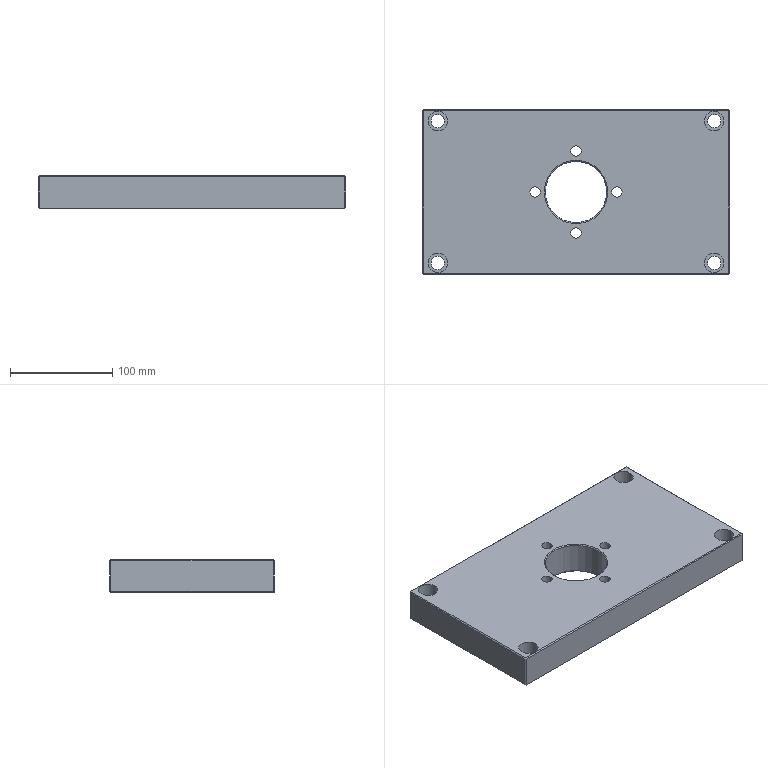Part | SolidWorks | features BaseBody 1 | 1 solid | 57 faces | box 300 x 160.5 x 32 mm | volume 1414203 mm3 | plane 27 | cylinder 26 | cone 4 | commonest cylinder face diameters 10.106 x8 13 x8 19 x8 60 x2